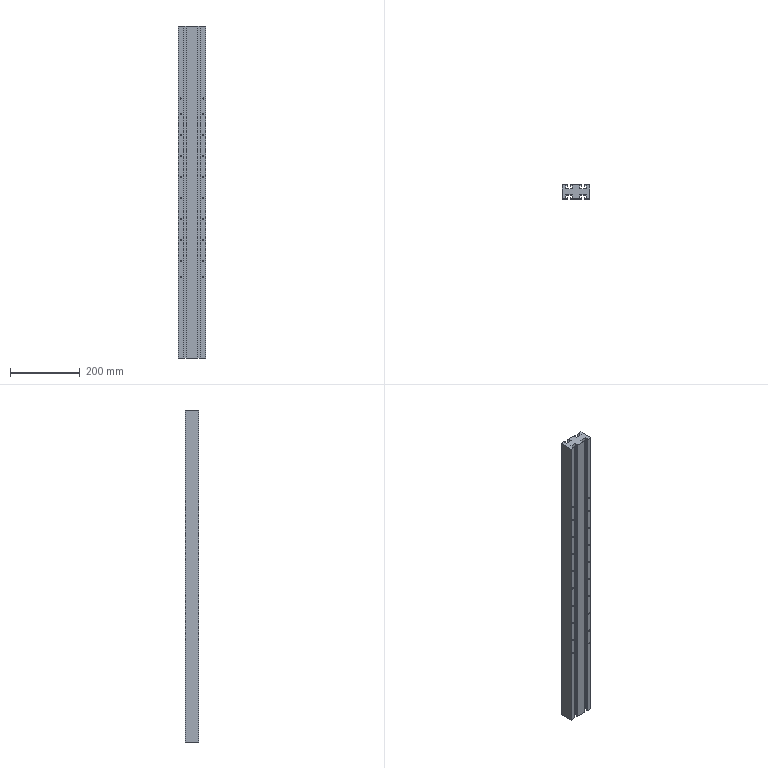Part | 1 solid | 172 faces | box 80 x 40 x 950 mm | volume 2352332 mm3 | cylinder 76 | plane 56 | cone 40 | commonest cylinder face diameters 3.3 x40 3.641 x32 16 x4